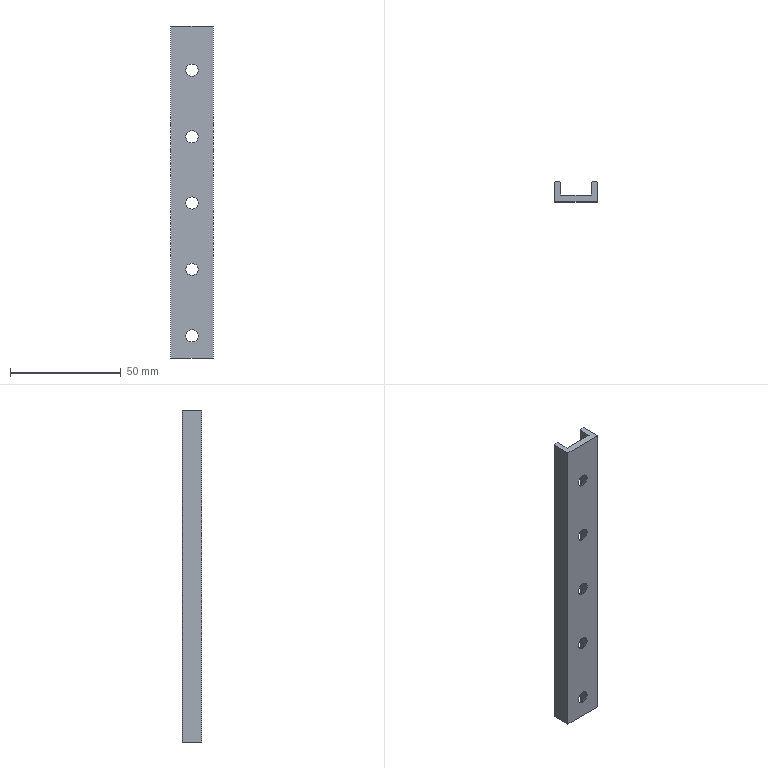Part | SolidWorks | features Chamfer 1, Extrusion 1, HoleWzd 1, LPattern 1 | 1 solid | 34 faces | box 19 x 9 x 150 mm | volume 12195 mm3 | plane 14 | cone 10 | cylinder 10 | commonest cylinder face diameters 5.5 x10
STEP:
#1=CARTESIAN_POINT('',(0.,-4.35,127.25));
#2=VERTEX_POINT('',#1);
#3=CARTESIAN_POINT('',(0.,-4.35,132.75));
#4=VERTEX_POINT('',#3);
#5=CARTESIAN_POINT('',(0.,-4.35,130.));
#6=DIRECTION('',(0.,1.,0.));
#7=DIRECTION('',(0.,0.,1.));
#8=AXIS2_PLACEMENT_3D('',#5,#6,#7);
#9=CIRCLE('',#8,2.75);
#10=EDGE_CURVE('',#2,#4,#9,.T.);
#11=ORIENTED_EDGE('',*,*,#10,.F.);
#12=CARTESIAN_POINT('',(0.,-1.5,124.4));
#13=VERTEX_POINT('',#12);
#14=CARTESIAN_POINT('',(0.,-1.5,124.4));
#15=DIRECTION('',(0.,0.7071,-0.7071));
#16=VECTOR('',#15,1000.);
#17=LINE('',#14,#16);
#18=EDGE_CURVE('',#2,#13,#17,.T.);
#19=ORIENTED_EDGE('',*,*,#18,.T.);
#20=CARTESIAN_POINT('',(0.,-1.5,135.6));
#21=VERTEX_POINT('',#20);
#22=CARTESIAN_POINT('',(0.,-1.5,130.));
#23=DIRECTION('',(0.,1.,0.));
#24=DIRECTION('',(0.,0.,1.));
#25=AXIS2_PLACEMENT_3D('',#22,#23,#24);
#26=CIRCLE('',#25,5.6);
#27=EDGE_CURVE('',#13,#21,#26,.T.);
#28=ORIENTED_EDGE('',*,*,#27,.T.);
#29=CARTESIAN_POINT('',(0.,-1.5,135.6));
#30=DIRECTION('',(0.,0.7071,0.7071));
#31=VECTOR('',#30,1000.);
#32=LINE('',#29,#31);
#33=EDGE_CURVE('',#4,#21,#32,.T.);
#34=ORIENTED_EDGE('',*,*,#33,.F.);
#35=EDGE_LOOP('',(#11,#19,#28,#34));
#36=FACE_OUTER_BOUND('',#35,.T.);
#37=CARTESIAN_POINT('',(0.,-1.5,130.));
#38=DIRECTION('',(0.,1.,0.));
#39=DIRECTION('',(0.,0.,1.));
#40=AXIS2_PLACEMENT_3D('',#37,#38,#39);
#41=CONICAL_SURFACE('',#40,5.6,0.7854);
#42=ADVANCED_FACE('',(#36),#41,.F.);
#43=CARTESIAN_POINT('',(0.,-4.5,127.25));
#44=VERTEX_POINT('',#43);
#45=CARTESIAN_POINT('',(0.,-4.5,132.75));
#46=VERTEX_POINT('',#45);
#47=CARTESIAN_POINT('',(0.,-4.5,130.));
#48=DIRECTION('',(0.,1.,0.));
#49=DIRECTION('',(0.,0.,1.));
#50=AXIS2_PLACEMENT_3D('',#47,#48,#49);
#51=CIRCLE('',#50,2.75);
#52=EDGE_CURVE('',#44,#46,#51,.T.);
#53=ORIENTED_EDGE('',*,*,#52,.F.);
#54=CARTESIAN_POINT('',(0.,-1.5,127.25));
#55=DIRECTION('',(0.,1.,0.));
#56=VECTOR('',#55,1000.);
#57=LINE('',#54,#56);
#58=EDGE_CURVE('',#44,#2,#57,.T.);
#59=ORIENTED_EDGE('',*,*,#58,.T.);
#60=ORIENTED_EDGE('',*,*,#10,.T.);
#61=CARTESIAN_POINT('',(0.,-1.5,132.75));
#62=DIRECTION('',(0.,1.,0.));
#63=VECTOR('',#62,1000.);
#64=LINE('',#61,#63);
#65=EDGE_CURVE('',#46,#4,#64,.T.);
#66=ORIENTED_EDGE('',*,*,#65,.F.);
#67=EDGE_LOOP('',(#53,#59,#60,#66));
#68=FACE_OUTER_BOUND('',#67,.T.);
#69=CARTESIAN_POINT('',(0.,-1.5,130.));
#70=DIRECTION('',(0.,1.,0.));
#71=DIRECTION('',(0.,0.,1.));
#72=AXIS2_PLACEMENT_3D('',#69,#70,#71);
#73=CYLINDRICAL_SURFACE('',#72,2.75);
#74=ADVANCED_FACE('',(#68),#73,.F.);
#75=CARTESIAN_POINT('',(0.,-4.35,97.25));
#76=VERTEX_POINT('',#75);
#77=CARTESIAN_POINT('',(0.,-4.35,102.75));
#78=VERTEX_POINT('',#77);
#79=CARTESIAN_POINT('',(0.,-4.35,100.));
#80=DIRECTION('',(0.,1.,0.));
#81=DIRECTION('',(0.,0.,1.));
#82=AXIS2_PLACEMENT_3D('',#79,#80,#81);
#83=CIRCLE('',#82,2.75);
#84=EDGE_CURVE('',#76,#78,#83,.T.);
#85=ORIENTED_EDGE('',*,*,#84,.F.);
#86=CARTESIAN_POINT('',(0.,-1.5,94.4));
#87=VERTEX_POINT('',#86);
#88=CARTESIAN_POINT('',(0.,-1.5,94.4));
#89=DIRECTION('',(0.,0.7071,-0.7071));
#90=VECTOR('',#89,1000.);
#91=LINE('',#88,#90);
#92=EDGE_CURVE('',#76,#87,#91,.T.);
#93=ORIENTED_EDGE('',*,*,#92,.T.);
#94=CARTESIAN_POINT('',(0.,-1.5,105.6));
#95=VERTEX_POINT('',#94);
#96=CARTESIAN_POINT('',(0.,-1.5,100.));
#97=DIRECTION('',(0.,1.,0.));
#98=DIRECTION('',(0.,0.,1.));
#99=AXIS2_PLACEMENT_3D('',#96,#97,#98);
#100=CIRCLE('',#99,5.6);
#101=EDGE_CURVE('',#87,#95,#100,.T.);
#102=ORIENTED_EDGE('',*,*,#101,.T.);
#103=CARTESIAN_POINT('',(0.,-1.5,105.6));
#104=DIRECTION('',(0.,0.7071,0.7071));
#105=VECTOR('',#104,1000.);
#106=LINE('',#103,#105);
#107=EDGE_CURVE('',#78,#95,#106,.T.);
#108=ORIENTED_EDGE('',*,*,#107,.F.);
#109=EDGE_LOOP('',(#85,#93,#102,#108));
#110=FACE_OUTER_BOUND('',#109,.T.);
#111=CARTESIAN_POINT('',(0.,-1.5,100.));
#112=DIRECTION('',(0.,1.,0.));
#113=DIRECTION('',(0.,0.,1.));
#114=AXIS2_PLACEMENT_3D('',#111,#112,#113);
#115=CONICAL_SURFACE('',#114,5.6,0.7854);
#116=ADVANCED_FACE('',(#110),#115,.F.);
#117=CARTESIAN_POINT('',(0.,-4.5,97.25));
#118=VERTEX_POINT('',#117);
#119=CARTESIAN_POINT('',(0.,-4.5,102.75));
#120=VERTEX_POINT('',#119);
#121=CARTESIAN_POINT('',(0.,-4.5,100.));
#122=DIRECTION('',(0.,1.,0.));
#123=DIRECTION('',(0.,0.,1.));
#124=AXIS2_PLACEMENT_3D('',#121,#122,#123);
#125=CIRCLE('',#124,2.75);
#126=EDGE_CURVE('',#118,#120,#125,.T.);
#127=ORIENTED_EDGE('',*,*,#126,.F.);
#128=CARTESIAN_POINT('',(0.,-1.5,97.25));
#129=DIRECTION('',(0.,1.,0.));
#130=VECTOR('',#129,1000.);
#131=LINE('',#128,#130);
#132=EDGE_CURVE('',#118,#76,#131,.T.);
#133=ORIENTED_EDGE('',*,*,#132,.T.);
#134=ORIENTED_EDGE('',*,*,#84,.T.);
#135=CARTESIAN_POINT('',(0.,-1.5,102.75));
#136=DIRECTION('',(0.,1.,0.));
#137=VECTOR('',#136,1000.);
#138=LINE('',#135,#137);
#139=EDGE_CURVE('',#120,#78,#138,.T.);
#140=ORIENTED_EDGE('',*,*,#139,.F.);
#141=EDGE_LOOP('',(#127,#133,#134,#140));
#142=FACE_OUTER_BOUND('',#141,.T.);
#143=CARTESIAN_POINT('',(0.,-1.5,100.));
#144=DIRECTION('',(0.,1.,0.));
#145=DIRECTION('',(0.,0.,1.));
#146=AXIS2_PLACEMENT_3D('',#143,#144,#145);
#147=CYLINDRICAL_SURFACE('',#146,2.75);
#148=ADVANCED_FACE('',(#142),#147,.F.);
#149=CARTESIAN_POINT('',(0.,-4.35,67.25));
#150=VERTEX_POINT('',#149);
#151=CARTESIAN_POINT('',(0.,-4.35,72.75));
#152=VERTEX_POINT('',#151);
#153=CARTESIAN_POINT('',(0.,-4.35,70.));
#154=DIRECTION('',(0.,1.,0.));
#155=DIRECTION('',(0.,0.,1.));
#156=AXIS2_PLACEMENT_3D('',#153,#154,#155);
#157=CIRCLE('',#156,2.75);
#158=EDGE_CURVE('',#150,#152,#157,.T.);
#159=ORIENTED_EDGE('',*,*,#158,.F.);
#160=CARTESIAN_POINT('',(0.,-1.5,64.4));
#161=VERTEX_POINT('',#160);
#162=CARTESIAN_POINT('',(0.,-1.5,64.4));
#163=DIRECTION('',(0.,0.7071,-0.7071));
#164=VECTOR('',#163,1000.);
#165=LINE('',#162,#164);
#166=EDGE_CURVE('',#150,#161,#165,.T.);
#167=ORIENTED_EDGE('',*,*,#166,.T.);
#168=CARTESIAN_POINT('',(0.,-1.5,75.6));
#169=VERTEX_POINT('',#168);
#170=CARTESIAN_POINT('',(0.,-1.5,70.));
#171=DIRECTION('',(0.,1.,0.));
#172=DIRECTION('',(0.,0.,1.));
#173=AXIS2_PLACEMENT_3D('',#170,#171,#172);
#174=CIRCLE('',#173,5.6);
#175=EDGE_CURVE('',#161,#169,#174,.T.);
#176=ORIENTED_EDGE('',*,*,#175,.T.);
#177=CARTESIAN_POINT('',(0.,-1.5,75.6));
#178=DIRECTION('',(0.,0.7071,0.7071));
#179=VECTOR('',#178,1000.);
#180=LINE('',#177,#179);
#181=EDGE_CURVE('',#152,#169,#180,.T.);
#182=ORIENTED_EDGE('',*,*,#181,.F.);
#183=EDGE_LOOP('',(#159,#167,#176,#182));
#184=FACE_OUTER_BOUND('',#183,.T.);
#185=CARTESIAN_POINT('',(0.,-1.5,70.));
#186=DIRECTION('',(0.,1.,0.));
#187=DIRECTION('',(0.,0.,1.));
#188=AXIS2_PLACEMENT_3D('',#185,#186,#187);
#189=CONICAL_SURFACE('',#188,5.6,0.7854);
#190=ADVANCED_FACE('',(#184),#189,.F.);
#191=CARTESIAN_POINT('',(0.,-4.5,67.25));
#192=VERTEX_POINT('',#191);
#193=CARTESIAN_POINT('',(0.,-4.5,72.75));
#194=VERTEX_POINT('',#193);
#195=CARTESIAN_POINT('',(0.,-4.5,70.));
#196=DIRECTION('',(0.,1.,0.));
#197=DIRECTION('',(0.,0.,1.));
#198=AXIS2_PLACEMENT_3D('',#195,#196,#197);
#199=CIRCLE('',#198,2.75);
#200=EDGE_CURVE('',#192,#194,#199,.T.);
#201=ORIENTED_EDGE('',*,*,#200,.F.);
#202=CARTESIAN_POINT('',(0.,-1.5,67.25));
#203=DIRECTION('',(0.,1.,0.));
#204=VECTOR('',#203,1000.);
#205=LINE('',#202,#204);
#206=EDGE_CURVE('',#192,#150,#205,.T.);
#207=ORIENTED_EDGE('',*,*,#206,.T.);
#208=ORIENTED_EDGE('',*,*,#158,.T.);
#209=CARTESIAN_POINT('',(0.,-1.5,72.75));
#210=DIRECTION('',(0.,1.,0.));
#211=VECTOR('',#210,1000.);
#212=LINE('',#209,#211);
#213=EDGE_CURVE('',#194,#152,#212,.T.);
#214=ORIENTED_EDGE('',*,*,#213,.F.);
#215=EDGE_LOOP('',(#201,#207,#208,#214));
#216=FACE_OUTER_BOUND('',#215,.T.);
#217=CARTESIAN_POINT('',(0.,-1.5,70.));
#218=DIRECTION('',(0.,1.,0.));
#219=DIRECTION('',(0.,0.,1.));
#220=AXIS2_PLACEMENT_3D('',#217,#218,#219);
#221=CYLINDRICAL_SURFACE('',#220,2.75);
#222=ADVANCED_FACE('',(#216),#221,.F.);
#223=CARTESIAN_POINT('',(0.,-4.35,7.25));
#224=VERTEX_POINT('',#223);
#225=CARTESIAN_POINT('',(0.,-4.35,12.75));
#226=VERTEX_POINT('',#225);
#227=CARTESIAN_POINT('',(0.,-4.35,10.));
#228=DIRECTION('',(0.,1.,0.));
#229=DIRECTION('',(0.,0.,1.));
#230=AXIS2_PLACEMENT_3D('',#227,#228,#229);
#231=CIRCLE('',#230,2.75);
#232=EDGE_CURVE('',#224,#226,#231,.T.);
#233=ORIENTED_EDGE('',*,*,#232,.F.);
#234=CARTESIAN_POINT('',(0.,-1.5,4.4));
#235=VERTEX_POINT('',#234);
#236=CARTESIAN_POINT('',(0.,-1.5,4.4));
#237=DIRECTION('',(0.,0.7071,-0.7071));
#238=VECTOR('',#237,1000.);
#239=LINE('',#236,#238);
#240=EDGE_CURVE('',#224,#235,#239,.T.);
#241=ORIENTED_EDGE('',*,*,#240,.T.);
#242=CARTESIAN_POINT('',(0.,-1.5,15.6));
#243=VERTEX_POINT('',#242);
#244=CARTESIAN_POINT('',(0.,-1.5,10.));
#245=DIRECTION('',(0.,1.,0.));
#246=DIRECTION('',(0.,0.,1.));
#247=AXIS2_PLACEMENT_3D('',#244,#245,#246);
#248=CIRCLE('',#247,5.6);
#249=EDGE_CURVE('',#235,#243,#248,.T.);
#250=ORIENTED_EDGE('',*,*,#249,.T.);
#251=CARTESIAN_POINT('',(0.,-1.5,15.6));
#252=DIRECTION('',(0.,0.7071,0.7071));
#253=VECTOR('',#252,1000.);
#254=LINE('',#251,#253);
#255=EDGE_CURVE('',#226,#243,#254,.T.);
#256=ORIENTED_EDGE('',*,*,#255,.F.);
#257=EDGE_LOOP('',(#233,#241,#250,#256));
#258=FACE_OUTER_BOUND('',#257,.T.);
#259=CARTESIAN_POINT('',(0.,-1.5,10.));
#260=DIRECTION('',(0.,1.,0.));
#261=DIRECTION('',(0.,0.,1.));
#262=AXIS2_PLACEMENT_3D('',#259,#260,#261);
#263=CONICAL_SURFACE('',#262,5.6,0.7854);
#264=ADVANCED_FACE('',(#258),#263,.F.);
#265=CARTESIAN_POINT('',(0.,-4.5,7.25));
#266=VERTEX_POINT('',#265);
#267=CARTESIAN_POINT('',(0.,-4.5,12.75));
#268=VERTEX_POINT('',#267);
#269=CARTESIAN_POINT('',(0.,-4.5,10.));
#270=DIRECTION('',(0.,1.,0.));
#271=DIRECTION('',(0.,0.,1.));
#272=AXIS2_PLACEMENT_3D('',#269,#270,#271);
#273=CIRCLE('',#272,2.75);
#274=EDGE_CURVE('',#266,#268,#273,.T.);
#275=ORIENTED_EDGE('',*,*,#274,.F.);
#276=CARTESIAN_POINT('',(0.,-1.5,7.25));
#277=DIRECTION('',(0.,1.,0.));
#278=VECTOR('',#277,1000.);
#279=LINE('',#276,#278);
#280=EDGE_CURVE('',#266,#224,#279,.T.);
#281=ORIENTED_EDGE('',*,*,#280,.T.);
#282=ORIENTED_EDGE('',*,*,#232,.T.);
#283=CARTESIAN_POINT('',(0.,-1.5,12.75));
#284=DIRECTION('',(0.,1.,0.));
#285=VECTOR('',#284,1000.);
#286=LINE('',#283,#285);
#287=EDGE_CURVE('',#268,#226,#286,.T.);
#288=ORIENTED_EDGE('',*,*,#287,.F.);
#289=EDGE_LOOP('',(#275,#281,#282,#288));
#290=FACE_OUTER_BOUND('',#289,.T.);
#291=CARTESIAN_POINT('',(0.,-1.5,10.));
#292=DIRECTION('',(0.,1.,0.));
#293=DIRECTION('',(0.,0.,1.));
#294=AXIS2_PLACEMENT_3D('',#291,#292,#293);
#295=CYLINDRICAL_SURFACE('',#294,2.75);
#296=ADVANCED_FACE('',(#290),#295,.F.);
#297=CARTESIAN_POINT('',(0.,-4.35,37.25));
#298=VERTEX_POINT('',#297);
#299=CARTESIAN_POINT('',(0.,-4.35,42.75));
#300=VERTEX_POINT('',#299);
#301=CARTESIAN_POINT('',(0.,-4.35,40.));
#302=DIRECTION('',(0.,1.,0.));
#303=DIRECTION('',(0.,0.,1.));
#304=AXIS2_PLACEMENT_3D('',#301,#302,#303);
#305=CIRCLE('',#304,2.75);
#306=EDGE_CURVE('',#298,#300,#305,.T.);
#307=ORIENTED_EDGE('',*,*,#306,.F.);
#308=CARTESIAN_POINT('',(0.,-1.5,34.4));
#309=VERTEX_POINT('',#308);
#310=CARTESIAN_POINT('',(0.,-1.5,34.4));
#311=DIRECTION('',(0.,0.7071,-0.7071));
#312=VECTOR('',#311,1000.);
#313=LINE('',#310,#312);
#314=EDGE_CURVE('',#298,#309,#313,.T.);
#315=ORIENTED_EDGE('',*,*,#314,.T.);
#316=CARTESIAN_POINT('',(0.,-1.5,45.6));
#317=VERTEX_POINT('',#316);
#318=CARTESIAN_POINT('',(0.,-1.5,40.));
#319=DIRECTION('',(0.,1.,0.));
#320=DIRECTION('',(0.,0.,1.));
#321=AXIS2_PLACEMENT_3D('',#318,#319,#320);
#322=CIRCLE('',#321,5.6);
#323=EDGE_CURVE('',#309,#317,#322,.T.);
#324=ORIENTED_EDGE('',*,*,#323,.T.);
#325=CARTESIAN_POINT('',(0.,-1.5,45.6));
#326=DIRECTION('',(0.,0.7071,0.7071));
#327=VECTOR('',#326,1000.);
#328=LINE('',#325,#327);
#329=EDGE_CURVE('',#300,#317,#328,.T.);
#330=ORIENTED_EDGE('',*,*,#329,.F.);
#331=EDGE_LOOP('',(#307,#315,#324,#330));
#332=FACE_OUTER_BOUND('',#331,.T.);
#333=CARTESIAN_POINT('',(0.,-1.5,40.));
#334=DIRECTION('',(0.,1.,0.));
#335=DIRECTION('',(0.,0.,1.));
#336=AXIS2_PLACEMENT_3D('',#333,#334,#335);
#337=CONICAL_SURFACE('',#336,5.6,0.7854);
#338=ADVANCED_FACE('',(#332),#337,.F.);
#339=CARTESIAN_POINT('',(0.,-4.5,37.25));
#340=VERTEX_POINT('',#339);
#341=CARTESIAN_POINT('',(0.,-4.5,42.75));
#342=VERTEX_POINT('',#341);
#343=CARTESIAN_POINT('',(0.,-4.5,40.));
#344=DIRECTION('',(0.,1.,0.));
#345=DIRECTION('',(0.,0.,1.));
#346=AXIS2_PLACEMENT_3D('',#343,#344,#345);
#347=CIRCLE('',#346,2.75);
#348=EDGE_CURVE('',#340,#342,#347,.T.);
#349=ORIENTED_EDGE('',*,*,#348,.F.);
#350=CARTESIAN_POINT('',(0.,-1.5,37.25));
#351=DIRECTION('',(0.,1.,0.));
#352=VECTOR('',#351,1000.);
#353=LINE('',#350,#352);
#354=EDGE_CURVE('',#340,#298,#353,.T.);
#355=ORIENTED_EDGE('',*,*,#354,.T.);
#356=ORIENTED_EDGE('',*,*,#306,.T.);
#357=CARTESIAN_POINT('',(0.,-1.5,42.75));
#358=DIRECTION('',(0.,1.,0.));
#359=VECTOR('',#358,1000.);
#360=LINE('',#357,#359);
#361=EDGE_CURVE('',#342,#300,#360,.T.);
#362=ORIENTED_EDGE('',*,*,#361,.F.);
#363=EDGE_LOOP('',(#349,#355,#356,#362));
#364=FACE_OUTER_BOUND('',#363,.T.);
#365=CARTESIAN_POINT('',(0.,-1.5,40.));
#366=DIRECTION('',(0.,1.,0.));
#367=DIRECTION('',(0.,0.,1.));
#368=AXIS2_PLACEMENT_3D('',#365,#366,#367);
#369=CYLINDRICAL_SURFACE('',#368,2.75);
#370=ADVANCED_FACE('',(#364),#369,.F.);
#371=CARTESIAN_POINT('',(9.2,4.5,150.));
#372=VERTEX_POINT('',#371);
#373=CARTESIAN_POINT('',(7.3,4.5,150.));
#374=VERTEX_POINT('',#373);
#375=CARTESIAN_POINT('',(7.,4.5,150.));
#376=DIRECTION('',(-1.,0.,0.));
#377=VECTOR('',#376,1000.);
#378=LINE('',#375,#377);
#379=EDGE_CURVE('',#372,#374,#378,.T.);
#380=ORIENTED_EDGE('',*,*,#379,.F.);
#381=CARTESIAN_POINT('',(9.2,4.5,0.));
#382=VERTEX_POINT('',#381);
#383=CARTESIAN_POINT('',(9.2,4.5,150.));
#384=DIRECTION('',(0.,0.,-1.));
#385=VECTOR('',#384,1000.);
#386=LINE('',#383,#385);
#387=EDGE_CURVE('',#372,#382,#386,.T.);
#388=ORIENTED_EDGE('',*,*,#387,.T.);
#389=CARTESIAN_POINT('',(7.3,4.5,0.));
#390=VERTEX_POINT('',#389);
#391=CARTESIAN_POINT('',(7.,4.5,0.));
#392=DIRECTION('',(-1.,0.,0.));
#393=VECTOR('',#392,1000.);
#394=LINE('',#391,#393);
#395=EDGE_CURVE('',#382,#390,#394,.T.);
#396=ORIENTED_EDGE('',*,*,#395,.T.);
#397=CARTESIAN_POINT('',(7.3,4.5,150.));
#398=DIRECTION('',(0.,0.,1.));
#399=VECTOR('',#398,1000.);
#400=LINE('',#397,#399);
#401=EDGE_CURVE('',#390,#374,#400,.T.);
#402=ORIENTED_EDGE('',*,*,#401,.T.);
#403=EDGE_LOOP('',(#380,#388,#396,#402));
#404=FACE_OUTER_BOUND('',#403,.T.);
#405=CARTESIAN_POINT('',(7.,4.5,150.));
#406=DIRECTION('',(0.,-1.,0.));
#407=DIRECTION('',(1.,0.,0.));
#408=AXIS2_PLACEMENT_3D('',#405,#406,#407);
#409=PLANE('',#408);
#410=ADVANCED_FACE('',(#404),#409,.F.);
#411=CARTESIAN_POINT('',(7.,4.2,150.));
#412=VERTEX_POINT('',#411);
#413=CARTESIAN_POINT('',(7.,-1.5,150.));
#414=VERTEX_POINT('',#413);
#415=CARTESIAN_POINT('',(7.,-1.5,150.));
#416=DIRECTION('',(0.,-1.,0.));
#417=VECTOR('',#416,1000.);
#418=LINE('',#415,#417);
#419=EDGE_CURVE('',#412,#414,#418,.T.);
#420=ORIENTED_EDGE('',*,*,#419,.F.);
#421=CARTESIAN_POINT('',(7.,4.2,0.));
#422=VERTEX_POINT('',#421);
#423=CARTESIAN_POINT('',(7.,4.2,150.));
#424=DIRECTION('',(0.,0.,-1.));
#425=VECTOR('',#424,1000.);
#426=LINE('',#423,#425);
#427=EDGE_CURVE('',#412,#422,#426,.T.);
#428=ORIENTED_EDGE('',*,*,#427,.T.);
#429=CARTESIAN_POINT('',(7.,-1.5,0.));
#430=VERTEX_POINT('',#429);
#431=CARTESIAN_POINT('',(7.,-1.5,0.));
#432=DIRECTION('',(0.,-1.,0.));
#433=VECTOR('',#432,1000.);
#434=LINE('',#431,#433);
#435=EDGE_CURVE('',#422,#430,#434,.T.);
#436=ORIENTED_EDGE('',*,*,#435,.T.);
#437=CARTESIAN_POINT('',(7.,-1.5,150.));
#438=DIRECTION('',(0.,0.,-1.));
#439=VECTOR('',#438,1000.);
#440=LINE('',#437,#439);
#441=EDGE_CURVE('',#414,#430,#440,.T.);
#442=ORIENTED_EDGE('',*,*,#441,.F.);
#443=EDGE_LOOP('',(#420,#428,#436,#442));
#444=FACE_OUTER_BOUND('',#443,.T.);
#445=CARTESIAN_POINT('',(7.,-1.5,150.));
#446=DIRECTION('',(1.,0.,0.));
#447=DIRECTION('',(0.,1.,0.));
#448=AXIS2_PLACEMENT_3D('',#445,#446,#447);
#449=PLANE('',#448);
#450=ADVANCED_FACE('',(#444),#449,.F.);
#451=CARTESIAN_POINT('',(0.,-1.5,130.));
#452=DIRECTION('',(0.,1.,0.));
#453=DIRECTION('',(0.,0.,1.));
#454=AXIS2_PLACEMENT_3D('',#451,#452,#453);
#455=CIRCLE('',#454,5.6);
#456=EDGE_CURVE('',#21,#13,#455,.T.);
#457=ORIENTED_EDGE('',*,*,#456,.F.);
#458=ORIENTED_EDGE('',*,*,#27,.F.);
#459=EDGE_LOOP('',(#457,#458));
#460=FACE_BOUND('',#459,.T.);
#461=CARTESIAN_POINT('',(0.,-1.5,100.));
#462=DIRECTION('',(0.,1.,0.));
#463=DIRECTION('',(0.,0.,1.));
#464=AXIS2_PLACEMENT_3D('',#461,#462,#463);
#465=CIRCLE('',#464,5.6);
#466=EDGE_CURVE('',#95,#87,#465,.T.);
#467=ORIENTED_EDGE('',*,*,#466,.F.);
#468=ORIENTED_EDGE('',*,*,#101,.F.);
#469=EDGE_LOOP('',(#467,#468));
#470=FACE_BOUND('',#469,.T.);
#471=CARTESIAN_POINT('',(0.,-1.5,70.));
#472=DIRECTION('',(0.,1.,0.));
#473=DIRECTION('',(0.,0.,1.));
#474=AXIS2_PLACEMENT_3D('',#471,#472,#473);
#475=CIRCLE('',#474,5.6);
#476=EDGE_CURVE('',#169,#161,#475,.T.);
#477=ORIENTED_EDGE('',*,*,#476,.F.);
#478=ORIENTED_EDGE('',*,*,#175,.F.);
#479=EDGE_LOOP('',(#477,#478));
#480=FACE_BOUND('',#479,.T.);
#481=CARTESIAN_POINT('',(0.,-1.5,10.));
#482=DIRECTION('',(0.,1.,0.));
#483=DIRECTION('',(0.,0.,1.));
#484=AXIS2_PLACEMENT_3D('',#481,#482,#483);
#485=CIRCLE('',#484,5.6);
#486=EDGE_CURVE('',#243,#235,#485,.T.);
#487=ORIENTED_EDGE('',*,*,#486,.F.);
#488=ORIENTED_EDGE('',*,*,#249,.F.);
#489=EDGE_LOOP('',(#487,#488));
#490=FACE_BOUND('',#489,.T.);
#491=CARTESIAN_POINT('',(0.,-1.5,40.));
#492=DIRECTION('',(0.,1.,0.));
#493=DIRECTION('',(0.,0.,1.));
#494=AXIS2_PLACEMENT_3D('',#491,#492,#493);
#495=CIRCLE('',#494,5.6);
#496=EDGE_CURVE('',#317,#309,#495,.T.);
#497=ORIENTED_EDGE('',*,*,#496,.F.);
#498=ORIENTED_EDGE('',*,*,#323,.F.);
#499=EDGE_LOOP('',(#497,#498));
#500=FACE_BOUND('',#499,.T.);
#501=CARTESIAN_POINT('',(-7.,-1.5,0.));
#502=VERTEX_POINT('',#501);
#503=CARTESIAN_POINT('',(-7.,-1.5,0.));
#504=DIRECTION('',(-1.,0.,0.));
#505=VECTOR('',#504,1000.);
#506=LINE('',#503,#505);
#507=EDGE_CURVE('',#430,#502,#506,.T.);
#508=ORIENTED_EDGE('',*,*,#507,.T.);
#509=CARTESIAN_POINT('',(-7.,-1.5,150.));
#510=VERTEX_POINT('',#509);
#511=CARTESIAN_POINT('',(-7.,-1.5,150.));
#512=DIRECTION('',(0.,0.,-1.));
#513=VECTOR('',#512,1000.);
#514=LINE('',#511,#513);
#515=EDGE_CURVE('',#510,#502,#514,.T.);
#516=ORIENTED_EDGE('',*,*,#515,.F.);
#517=CARTESIAN_POINT('',(-7.,-1.5,150.));
#518=DIRECTION('',(-1.,0.,0.));
#519=VECTOR('',#518,1000.);
#520=LINE('',#517,#519);
#521=EDGE_CURVE('',#414,#510,#520,.T.);
#522=ORIENTED_EDGE('',*,*,#521,.F.);
#523=ORIENTED_EDGE('',*,*,#441,.T.);
#524=EDGE_LOOP('',(#508,#516,#522,#523));
#525=FACE_OUTER_BOUND('',#524,.T.);
#526=CARTESIAN_POINT('',(-7.,-1.5,150.));
#527=DIRECTION('',(0.,-1.,0.));
#528=DIRECTION('',(1.,0.,0.));
#529=AXIS2_PLACEMENT_3D('',#526,#527,#528);
#530=PLANE('',#529);
#531=ADVANCED_FACE('',(#460,#470,#480,#490,#500,#525),#530,.F.);
#532=CARTESIAN_POINT('',(-7.,4.2,0.));
#533=VERTEX_POINT('',#532);
#534=CARTESIAN_POINT('',(-7.,4.5,0.));
#535=DIRECTION('',(0.,1.,0.));
#536=VECTOR('',#535,1000.);
#537=LINE('',#534,#536);
#538=EDGE_CURVE('',#502,#533,#537,.T.);
#539=ORIENTED_EDGE('',*,*,#538,.T.);
#540=CARTESIAN_POINT('',(-7.,4.2,150.));
#541=VERTEX_POINT('',#540);
#542=CARTESIAN_POINT('',(-7.,4.2,150.));
#543=DIRECTION('',(0.,0.,1.));
#544=VECTOR('',#543,1000.);
#545=LINE('',#542,#544);
#546=EDGE_CURVE('',#533,#541,#545,.T.);
#547=ORIENTED_EDGE('',*,*,#546,.T.);
#548=CARTESIAN_POINT('',(-7.,4.5,150.));
#549=DIRECTION('',(0.,1.,0.));
#550=VECTOR('',#549,1000.);
#551=LINE('',#548,#550);
#552=EDGE_CURVE('',#510,#541,#551,.T.);
#553=ORIENTED_EDGE('',*,*,#552,.F.);
#554=ORIENTED_EDGE('',*,*,#515,.T.);
#555=EDGE_LOOP('',(#539,#547,#553,#554));
#556=FACE_OUTER_BOUND('',#555,.T.);
#557=CARTESIAN_POINT('',(-7.,4.5,150.));
#558=DIRECTION('',(-1.,0.,0.));
#559=DIRECTION('',(0.,-1.,0.));
#560=AXIS2_PLACEMENT_3D('',#557,#558,#559);
#561=PLANE('',#560);
#562=ADVANCED_FACE('',(#556),#561,.F.);
#563=CARTESIAN_POINT('',(-7.3,4.5,0.));
#564=VERTEX_POINT('',#563);
#565=CARTESIAN_POINT('',(-9.2,4.5,0.));
#566=VERTEX_POINT('',#565);
#567=CARTESIAN_POINT('',(-9.5,4.5,0.));
#568=DIRECTION('',(-1.,0.,0.));
#569=VECTOR('',#568,1000.);
#570=LINE('',#567,#569);
#571=EDGE_CURVE('',#564,#566,#570,.T.);
#572=ORIENTED_EDGE('',*,*,#571,.T.);
#573=CARTESIAN_POINT('',(-9.2,4.5,150.));
#574=VERTEX_POINT('',#573);
#575=CARTESIAN_POINT('',(-9.2,4.5,150.));
#576=DIRECTION('',(0.,0.,1.));
#577=VECTOR('',#576,1000.);
#578=LINE('',#575,#577);
#579=EDGE_CURVE('',#566,#574,#578,.T.);
#580=ORIENTED_EDGE('',*,*,#579,.T.);
#581=CARTESIAN_POINT('',(-7.3,4.5,150.));
#582=VERTEX_POINT('',#581);
#583=CARTESIAN_POINT('',(-9.5,4.5,150.));
#584=DIRECTION('',(-1.,0.,0.));
#585=VECTOR('',#584,1000.);
#586=LINE('',#583,#585);
#587=EDGE_CURVE('',#582,#574,#586,.T.);
#588=ORIENTED_EDGE('',*,*,#587,.F.);
#589=CARTESIAN_POINT('',(-7.3,4.5,150.));
#590=DIRECTION('',(0.,0.,-1.));
#591=VECTOR('',#590,1000.);
#592=LINE('',#589,#591);
#593=EDGE_CURVE('',#582,#564,#592,.T.);
#594=ORIENTED_EDGE('',*,*,#593,.T.);
#595=EDGE_LOOP('',(#572,#580,#588,#594));
#596=FACE_OUTER_BOUND('',#595,.T.);
#597=CARTESIAN_POINT('',(-9.5,4.5,150.));
#598=DIRECTION('',(0.,-1.,0.));
#599=DIRECTION('',(1.,0.,0.));
#600=AXIS2_PLACEMENT_3D('',#597,#598,#599);
#601=PLANE('',#600);
#602=ADVANCED_FACE('',(#596),#601,.F.);
#603=CARTESIAN_POINT('',(-9.5,4.2,150.));
#604=VERTEX_POINT('',#603);
#605=CARTESIAN_POINT('',(-9.5,-4.5,150.));
#606=VERTEX_POINT('',#605);
#607=CARTESIAN_POINT('',(-9.5,-4.5,150.));
#608=DIRECTION('',(0.,-1.,0.));
#609=VECTOR('',#608,1000.);
#610=LINE('',#607,#609);
#611=EDGE_CURVE('',#604,#606,#610,.T.);
#612=ORIENTED_EDGE('',*,*,#611,.F.);
#613=CARTESIAN_POINT('',(-9.5,4.2,0.));
#614=VERTEX_POINT('',#613);
#615=CARTESIAN_POINT('',(-9.5,4.2,150.));
#616=DIRECTION('',(0.,0.,-1.));
#617=VECTOR('',#616,1000.);
#618=LINE('',#615,#617);
#619=EDGE_CURVE('',#604,#614,#618,.T.);
#620=ORIENTED_EDGE('',*,*,#619,.T.);
#621=CARTESIAN_POINT('',(-9.5,-4.5,0.));
#622=VERTEX_POINT('',#621);
#623=CARTESIAN_POINT('',(-9.5,-4.5,0.));
#624=DIRECTION('',(0.,-1.,0.));
#625=VECTOR('',#624,1000.);
#626=LINE('',#623,#625);
#627=EDGE_CURVE('',#614,#622,#626,.T.);
#628=ORIENTED_EDGE('',*,*,#627,.T.);
#629=CARTESIAN_POINT('',(-9.5,-4.5,150.));
#630=DIRECTION('',(0.,0.,-1.));
#631=VECTOR('',#630,1000.);
#632=LINE('',#629,#631);
#633=EDGE_CURVE('',#606,#622,#632,.T.);
#634=ORIENTED_EDGE('',*,*,#633,.F.);
#635=EDGE_LOOP('',(#612,#620,#628,#634));
#636=FACE_OUTER_BOUND('',#635,.T.);
#637=CARTESIAN_POINT('',(-9.5,-4.5,150.));
#638=DIRECTION('',(1.,0.,0.));
#639=DIRECTION('',(0.,0.,-1.));
#640=AXIS2_PLACEMENT_3D('',#637,#638,#639);
#641=PLANE('',#640);
#642=ADVANCED_FACE('',(#636),#641,.F.);
#643=CARTESIAN_POINT('',(0.,-4.5,130.));
#644=DIRECTION('',(0.,1.,0.));
#645=DIRECTION('',(0.,0.,1.));
#646=AXIS2_PLACEMENT_3D('',#643,#644,#645);
#647=CIRCLE('',#646,2.75);
#648=EDGE_CURVE('',#46,#44,#647,.T.);
#649=ORIENTED_EDGE('',*,*,#648,.T.);
#650=ORIENTED_EDGE('',*,*,#52,.T.);
#651=EDGE_LOOP('',(#649,#650));
#652=FACE_BOUND('',#651,.T.);
#653=CARTESIAN_POINT('',(0.,-4.5,100.));
#654=DIRECTION('',(0.,1.,0.));
#655=DIRECTION('',(0.,0.,1.));
#656=AXIS2_PLACEMENT_3D('',#653,#654,#655);
#657=CIRCLE('',#656,2.75);
#658=EDGE_CURVE('',#120,#118,#657,.T.);
#659=ORIENTED_EDGE('',*,*,#658,.T.);
#660=ORIENTED_EDGE('',*,*,#126,.T.);
#661=EDGE_LOOP('',(#659,#660));
#662=FACE_BOUND('',#661,.T.);
#663=CARTESIAN_POINT('',(0.,-4.5,70.));
#664=DIRECTION('',(0.,1.,0.));
#665=DIRECTION('',(0.,0.,1.));
#666=AXIS2_PLACEMENT_3D('',#663,#664,#665);
#667=CIRCLE('',#666,2.75);
#668=EDGE_CURVE('',#194,#192,#667,.T.);
#669=ORIENTED_EDGE('',*,*,#668,.T.);
#670=ORIENTED_EDGE('',*,*,#200,.T.);
#671=EDGE_LOOP('',(#669,#670));
#672=FACE_BOUND('',#671,.T.);
#673=CARTESIAN_POINT('',(0.,-4.5,10.));
#674=DIRECTION('',(0.,1.,0.));
#675=DIRECTION('',(0.,0.,1.));
#676=AXIS2_PLACEMENT_3D('',#673,#674,#675);
#677=CIRCLE('',#676,2.75);
#678=EDGE_CURVE('',#268,#266,#677,.T.);
#679=ORIENTED_EDGE('',*,*,#678,.T.);
#680=ORIENTED_EDGE('',*,*,#274,.T.);
#681=EDGE_LOOP('',(#679,#680));
#682=FACE_BOUND('',#681,.T.);
#683=CARTESIAN_POINT('',(0.,-4.5,40.));
#684=DIRECTION('',(0.,1.,0.));
#685=DIRECTION('',(0.,0.,1.));
#686=AXIS2_PLACEMENT_3D('',#683,#684,#685);
#687=CIRCLE('',#686,2.75);
#688=EDGE_CURVE('',#342,#340,#687,.T.);
#689=ORIENTED_EDGE('',*,*,#688,.T.);
#690=ORIENTED_EDGE('',*,*,#348,.T.);
#691=EDGE_LOOP('',(#689,#690));
#692=FACE_BOUND('',#691,.T.);
#693=CARTESIAN_POINT('',(9.5,-4.5,0.));
#694=VERTEX_POINT('',#693);
#695=CARTESIAN_POINT('',(-9.5,-4.5,0.));
#696=DIRECTION('',(1.,0.,0.));
#697=VECTOR('',#696,1000.);
#698=LINE('',#695,#697);
#699=EDGE_CURVE('',#622,#694,#698,.T.);
#700=ORIENTED_EDGE('',*,*,#699,.T.);
#701=CARTESIAN_POINT('',(9.5,-4.5,150.));
#702=VERTEX_POINT('',#701);
#703=CARTESIAN_POINT('',(9.5,-4.5,150.));
#704=DIRECTION('',(0.,0.,-1.));
#705=VECTOR('',#704,1000.);
#706=LINE('',#703,#705);
#707=EDGE_CURVE('',#702,#694,#706,.T.);
#708=ORIENTED_EDGE('',*,*,#707,.F.);
#709=CARTESIAN_POINT('',(-9.5,-4.5,150.));
#710=DIRECTION('',(1.,0.,0.));
#711=VECTOR('',#710,1000.);
#712=LINE('',#709,#711);
#713=EDGE_CURVE('',#606,#702,#712,.T.);
#714=ORIENTED_EDGE('',*,*,#713,.F.);
#715=ORIENTED_EDGE('',*,*,#633,.T.);
#716=EDGE_LOOP('',(#700,#708,#714,#715));
#717=FACE_OUTER_BOUND('',#716,.T.);
#718=CARTESIAN_POINT('',(-9.5,-4.5,150.));
#719=DIRECTION('',(0.,1.,0.));
#720=DIRECTION('',(0.,0.,1.));
#721=AXIS2_PLACEMENT_3D('',#718,#719,#720);
#722=PLANE('',#721);
#723=ADVANCED_FACE('',(#652,#662,#672,#682,#692,#717),#722,.F.);
#724=CARTESIAN_POINT('',(9.5,4.2,0.));
#725=VERTEX_POINT('',#724);
#726=CARTESIAN_POINT('',(9.5,-4.5,0.));
#727=DIRECTION('',(0.,1.,0.));
#728=VECTOR('',#727,1000.);
#729=LINE('',#726,#728);
#730=EDGE_CURVE('',#694,#725,#729,.T.);
#731=ORIENTED_EDGE('',*,*,#730,.T.);
#732=CARTESIAN_POINT('',(9.5,4.2,150.));
#733=VERTEX_POINT('',#732);
#734=CARTESIAN_POINT('',(9.5,4.2,150.));
#735=DIRECTION('',(0.,0.,1.));
#736=VECTOR('',#735,1000.);
#737=LINE('',#734,#736);
#738=EDGE_CURVE('',#725,#733,#737,.T.);
#739=ORIENTED_EDGE('',*,*,#738,.T.);
#740=CARTESIAN_POINT('',(9.5,-4.5,150.));
#741=DIRECTION('',(0.,1.,0.));
#742=VECTOR('',#741,1000.);
#743=LINE('',#740,#742);
#744=EDGE_CURVE('',#702,#733,#743,.T.);
#745=ORIENTED_EDGE('',*,*,#744,.F.);
#746=ORIENTED_EDGE('',*,*,#707,.T.);
#747=EDGE_LOOP('',(#731,#739,#745,#746));
#748=FACE_OUTER_BOUND('',#747,.T.);
#749=CARTESIAN_POINT('',(9.5,-4.5,150.));
#750=DIRECTION('',(-1.,0.,0.));
#751=DIRECTION('',(0.,0.,1.));
#752=AXIS2_PLACEMENT_3D('',#749,#750,#751);
#753=PLANE('',#752);
#754=ADVANCED_FACE('',(#748),#753,.F.);
#755=ORIENTED_EDGE('',*,*,#587,.T.);
#756=CARTESIAN_POINT('',(-6.85,6.85,150.));
#757=DIRECTION('',(-0.7071,-0.7071,0.));
#758=VECTOR('',#757,1000.);
#759=LINE('',#756,#758);
#760=EDGE_CURVE('',#574,#604,#759,.T.);
#761=ORIENTED_EDGE('',*,*,#760,.T.);
#762=ORIENTED_EDGE('',*,*,#611,.T.);
#763=ORIENTED_EDGE('',*,*,#713,.T.);
#764=ORIENTED_EDGE('',*,*,#744,.T.);
#765=CARTESIAN_POINT('',(6.85,6.85,150.));
#766=DIRECTION('',(-0.7071,0.7071,0.));
#767=VECTOR('',#766,1000.);
#768=LINE('',#765,#767);
#769=EDGE_CURVE('',#733,#372,#768,.T.);
#770=ORIENTED_EDGE('',*,*,#769,.T.);
#771=ORIENTED_EDGE('',*,*,#379,.T.);
#772=CARTESIAN_POINT('',(1.4,-1.4,150.));
#773=DIRECTION('',(-0.7071,-0.7071,0.));
#774=VECTOR('',#773,1000.);
#775=LINE('',#772,#774);
#776=EDGE_CURVE('',#374,#412,#775,.T.);
#777=ORIENTED_EDGE('',*,*,#776,.T.);
#778=ORIENTED_EDGE('',*,*,#419,.T.);
#779=ORIENTED_EDGE('',*,*,#521,.T.);
#780=ORIENTED_EDGE('',*,*,#552,.T.);
#781=CARTESIAN_POINT('',(-1.4,-1.4,150.));
#782=DIRECTION('',(-0.7071,0.7071,0.));
#783=VECTOR('',#782,1000.);
#784=LINE('',#781,#783);
#785=EDGE_CURVE('',#541,#582,#784,.T.);
#786=ORIENTED_EDGE('',*,*,#785,.T.);
#787=EDGE_LOOP('',(#755,#761,#762,#763,#764,#770,#771,#777,#778,#779,#780,#786));
#788=FACE_OUTER_BOUND('',#787,.T.);
#789=CARTESIAN_POINT('',(0.,0.,150.));
#790=DIRECTION('',(0.,0.,1.));
#791=DIRECTION('',(1.,0.,0.));
#792=AXIS2_PLACEMENT_3D('',#789,#790,#791);
#793=PLANE('',#792);
#794=ADVANCED_FACE('',(#788),#793,.T.);
#795=ORIENTED_EDGE('',*,*,#627,.F.);
#796=CARTESIAN_POINT('',(-9.5,4.2,0.));
#797=DIRECTION('',(0.7071,0.7071,0.));
#798=VECTOR('',#797,1000.);
#799=LINE('',#796,#798);
#800=EDGE_CURVE('',#614,#566,#799,.T.);
#801=ORIENTED_EDGE('',*,*,#800,.T.);
#802=ORIENTED_EDGE('',*,*,#571,.F.);
#803=CARTESIAN_POINT('',(-7.3,4.5,0.));
#804=DIRECTION('',(0.7071,-0.7071,0.));
#805=VECTOR('',#804,1000.);
#806=LINE('',#803,#805);
#807=EDGE_CURVE('',#564,#533,#806,.T.);
#808=ORIENTED_EDGE('',*,*,#807,.T.);
#809=ORIENTED_EDGE('',*,*,#538,.F.);
#810=ORIENTED_EDGE('',*,*,#507,.F.);
#811=ORIENTED_EDGE('',*,*,#435,.F.);
#812=CARTESIAN_POINT('',(7.,4.2,0.));
#813=DIRECTION('',(0.7071,0.7071,0.));
#814=VECTOR('',#813,1000.);
#815=LINE('',#812,#814);
#816=EDGE_CURVE('',#422,#390,#815,.T.);
#817=ORIENTED_EDGE('',*,*,#816,.T.);
#818=ORIENTED_EDGE('',*,*,#395,.F.);
#819=CARTESIAN_POINT('',(9.2,4.5,0.));
#820=DIRECTION('',(0.7071,-0.7071,0.));
#821=VECTOR('',#820,1000.);
#822=LINE('',#819,#821);
#823=EDGE_CURVE('',#382,#725,#822,.T.);
#824=ORIENTED_EDGE('',*,*,#823,.T.);
#825=ORIENTED_EDGE('',*,*,#730,.F.);
#826=ORIENTED_EDGE('',*,*,#699,.F.);
#827=EDGE_LOOP('',(#795,#801,#802,#808,#809,#810,#811,#817,#818,#824,#825,#826));
#828=FACE_OUTER_BOUND('',#827,.T.);
#829=CARTESIAN_POINT('',(0.,0.,0.));
#830=DIRECTION('',(0.,0.,1.));
#831=DIRECTION('',(1.,0.,0.));
#832=AXIS2_PLACEMENT_3D('',#829,#830,#831);
#833=PLANE('',#832);
#834=ADVANCED_FACE('',(#828),#833,.F.);
#835=ORIENTED_EDGE('',*,*,#354,.F.);
#836=ORIENTED_EDGE('',*,*,#688,.F.);
#837=ORIENTED_EDGE('',*,*,#361,.T.);
#838=CARTESIAN_POINT('',(0.,-4.35,40.));
#839=DIRECTION('',(0.,1.,0.));
#840=DIRECTION('',(0.,0.,1.));
#841=AXIS2_PLACEMENT_3D('',#838,#839,#840);
#842=CIRCLE('',#841,2.75);
#843=EDGE_CURVE('',#300,#298,#842,.T.);
#844=ORIENTED_EDGE('',*,*,#843,.T.);
#845=EDGE_LOOP('',(#835,#836,#837,#844));
#846=FACE_OUTER_BOUND('',#845,.T.);
#847=CARTESIAN_POINT('',(0.,-1.5,40.));
#848=DIRECTION('',(0.,1.,0.));
#849=DIRECTION('',(0.,0.,1.));
#850=AXIS2_PLACEMENT_3D('',#847,#848,#849);
#851=CYLINDRICAL_SURFACE('',#850,2.75);
#852=ADVANCED_FACE('',(#846),#851,.F.);
#853=ORIENTED_EDGE('',*,*,#314,.F.);
#854=ORIENTED_EDGE('',*,*,#843,.F.);
#855=ORIENTED_EDGE('',*,*,#329,.T.);
#856=ORIENTED_EDGE('',*,*,#496,.T.);
#857=EDGE_LOOP('',(#853,#854,#855,#856));
#858=FACE_OUTER_BOUND('',#857,.T.);
#859=CARTESIAN_POINT('',(0.,-1.5,40.));
#860=DIRECTION('',(0.,1.,0.));
#861=DIRECTION('',(0.,0.,1.));
#862=AXIS2_PLACEMENT_3D('',#859,#860,#861);
#863=CONICAL_SURFACE('',#862,5.6,0.7854);
#864=ADVANCED_FACE('',(#858),#863,.F.);
#865=ORIENTED_EDGE('',*,*,#280,.F.);
#866=ORIENTED_EDGE('',*,*,#678,.F.);
#867=ORIENTED_EDGE('',*,*,#287,.T.);
#868=CARTESIAN_POINT('',(0.,-4.35,10.));
#869=DIRECTION('',(0.,1.,0.));
#870=DIRECTION('',(0.,0.,1.));
#871=AXIS2_PLACEMENT_3D('',#868,#869,#870);
#872=CIRCLE('',#871,2.75);
#873=EDGE_CURVE('',#226,#224,#872,.T.);
#874=ORIENTED_EDGE('',*,*,#873,.T.);
#875=EDGE_LOOP('',(#865,#866,#867,#874));
#876=FACE_OUTER_BOUND('',#875,.T.);
#877=CARTESIAN_POINT('',(0.,-1.5,10.));
#878=DIRECTION('',(0.,1.,0.));
#879=DIRECTION('',(0.,0.,1.));
#880=AXIS2_PLACEMENT_3D('',#877,#878,#879);
#881=CYLINDRICAL_SURFACE('',#880,2.75);
#882=ADVANCED_FACE('',(#876),#881,.F.);
#883=ORIENTED_EDGE('',*,*,#240,.F.);
#884=ORIENTED_EDGE('',*,*,#873,.F.);
#885=ORIENTED_EDGE('',*,*,#255,.T.);
#886=ORIENTED_EDGE('',*,*,#486,.T.);
#887=EDGE_LOOP('',(#883,#884,#885,#886));
#888=FACE_OUTER_BOUND('',#887,.T.);
#889=CARTESIAN_POINT('',(0.,-1.5,10.));
#890=DIRECTION('',(0.,1.,0.));
#891=DIRECTION('',(0.,0.,1.));
#892=AXIS2_PLACEMENT_3D('',#889,#890,#891);
#893=CONICAL_SURFACE('',#892,5.6,0.7854);
#894=ADVANCED_FACE('',(#888),#893,.F.);
#895=ORIENTED_EDGE('',*,*,#206,.F.);
#896=ORIENTED_EDGE('',*,*,#668,.F.);
#897=ORIENTED_EDGE('',*,*,#213,.T.);
#898=CARTESIAN_POINT('',(0.,-4.35,70.));
#899=DIRECTION('',(0.,1.,0.));
#900=DIRECTION('',(0.,0.,1.));
#901=AXIS2_PLACEMENT_3D('',#898,#899,#900);
#902=CIRCLE('',#901,2.75);
#903=EDGE_CURVE('',#152,#150,#902,.T.);
#904=ORIENTED_EDGE('',*,*,#903,.T.);
#905=EDGE_LOOP('',(#895,#896,#897,#904));
#906=FACE_OUTER_BOUND('',#905,.T.);
#907=CARTESIAN_POINT('',(0.,-1.5,70.));
#908=DIRECTION('',(0.,1.,0.));
#909=DIRECTION('',(0.,0.,1.));
#910=AXIS2_PLACEMENT_3D('',#907,#908,#909);
#911=CYLINDRICAL_SURFACE('',#910,2.75);
#912=ADVANCED_FACE('',(#906),#911,.F.);
#913=ORIENTED_EDGE('',*,*,#166,.F.);
#914=ORIENTED_EDGE('',*,*,#903,.F.);
#915=ORIENTED_EDGE('',*,*,#181,.T.);
#916=ORIENTED_EDGE('',*,*,#476,.T.);
#917=EDGE_LOOP('',(#913,#914,#915,#916));
#918=FACE_OUTER_BOUND('',#917,.T.);
#919=CARTESIAN_POINT('',(0.,-1.5,70.));
#920=DIRECTION('',(0.,1.,0.));
#921=DIRECTION('',(0.,0.,1.));
#922=AXIS2_PLACEMENT_3D('',#919,#920,#921);
#923=CONICAL_SURFACE('',#922,5.6,0.7854);
#924=ADVANCED_FACE('',(#918),#923,.F.);
#925=ORIENTED_EDGE('',*,*,#132,.F.);
#926=ORIENTED_EDGE('',*,*,#658,.F.);
#927=ORIENTED_EDGE('',*,*,#139,.T.);
#928=CARTESIAN_POINT('',(0.,-4.35,100.));
#929=DIRECTION('',(0.,1.,0.));
#930=DIRECTION('',(0.,0.,1.));
#931=AXIS2_PLACEMENT_3D('',#928,#929,#930);
#932=CIRCLE('',#931,2.75);
#933=EDGE_CURVE('',#78,#76,#932,.T.);
#934=ORIENTED_EDGE('',*,*,#933,.T.);
#935=EDGE_LOOP('',(#925,#926,#927,#934));
#936=FACE_OUTER_BOUND('',#935,.T.);
#937=CARTESIAN_POINT('',(0.,-1.5,100.));
#938=DIRECTION('',(0.,1.,0.));
#939=DIRECTION('',(0.,0.,1.));
#940=AXIS2_PLACEMENT_3D('',#937,#938,#939);
#941=CYLINDRICAL_SURFACE('',#940,2.75);
#942=ADVANCED_FACE('',(#936),#941,.F.);
#943=ORIENTED_EDGE('',*,*,#92,.F.);
#944=ORIENTED_EDGE('',*,*,#933,.F.);
#945=ORIENTED_EDGE('',*,*,#107,.T.);
#946=ORIENTED_EDGE('',*,*,#466,.T.);
#947=EDGE_LOOP('',(#943,#944,#945,#946));
#948=FACE_OUTER_BOUND('',#947,.T.);
#949=CARTESIAN_POINT('',(0.,-1.5,100.));
#950=DIRECTION('',(0.,1.,0.));
#951=DIRECTION('',(0.,0.,1.));
#952=AXIS2_PLACEMENT_3D('',#949,#950,#951);
#953=CONICAL_SURFACE('',#952,5.6,0.7854);
#954=ADVANCED_FACE('',(#948),#953,.F.);
#955=ORIENTED_EDGE('',*,*,#58,.F.);
#956=ORIENTED_EDGE('',*,*,#648,.F.);
#957=ORIENTED_EDGE('',*,*,#65,.T.);
#958=CARTESIAN_POINT('',(0.,-4.35,130.));
#959=DIRECTION('',(0.,1.,0.));
#960=DIRECTION('',(0.,0.,1.));
#961=AXIS2_PLACEMENT_3D('',#958,#959,#960);
#962=CIRCLE('',#961,2.75);
#963=EDGE_CURVE('',#4,#2,#962,.T.);
#964=ORIENTED_EDGE('',*,*,#963,.T.);
#965=EDGE_LOOP('',(#955,#956,#957,#964));
#966=FACE_OUTER_BOUND('',#965,.T.);
#967=CARTESIAN_POINT('',(0.,-1.5,130.));
#968=DIRECTION('',(0.,1.,0.));
#969=DIRECTION('',(0.,0.,1.));
#970=AXIS2_PLACEMENT_3D('',#967,#968,#969);
#971=CYLINDRICAL_SURFACE('',#970,2.75);
#972=ADVANCED_FACE('',(#966),#971,.F.);
#973=ORIENTED_EDGE('',*,*,#18,.F.);
#974=ORIENTED_EDGE('',*,*,#963,.F.);
#975=ORIENTED_EDGE('',*,*,#33,.T.);
#976=ORIENTED_EDGE('',*,*,#456,.T.);
#977=EDGE_LOOP('',(#973,#974,#975,#976));
#978=FACE_OUTER_BOUND('',#977,.T.);
#979=CARTESIAN_POINT('',(0.,-1.5,130.));
#980=DIRECTION('',(0.,1.,0.));
#981=DIRECTION('',(0.,0.,1.));
#982=AXIS2_PLACEMENT_3D('',#979,#980,#981);
#983=CONICAL_SURFACE('',#982,5.6,0.7854);
#984=ADVANCED_FACE('',(#978),#983,.F.);
#985=ORIENTED_EDGE('',*,*,#760,.F.);
#986=ORIENTED_EDGE('',*,*,#579,.F.);
#987=ORIENTED_EDGE('',*,*,#800,.F.);
#988=ORIENTED_EDGE('',*,*,#619,.F.);
#989=EDGE_LOOP('',(#985,#986,#987,#988));
#990=FACE_OUTER_BOUND('',#989,.T.);
#991=CARTESIAN_POINT('',(-9.5,4.2,150.));
#992=DIRECTION('',(0.7071,-0.7071,0.));
#993=DIRECTION('',(0.,0.,-1.));
#994=AXIS2_PLACEMENT_3D('',#991,#992,#993);
#995=PLANE('',#994);
#996=ADVANCED_FACE('',(#990),#995,.F.);
#997=ORIENTED_EDGE('',*,*,#769,.F.);
#998=ORIENTED_EDGE('',*,*,#738,.F.);
#999=ORIENTED_EDGE('',*,*,#823,.F.);
#1000=ORIENTED_EDGE('',*,*,#387,.F.);
#1001=EDGE_LOOP('',(#997,#998,#999,#1000));
#1002=FACE_OUTER_BOUND('',#1001,.T.);
#1003=CARTESIAN_POINT('',(9.2,4.5,150.));
#1004=DIRECTION('',(-0.7071,-0.7071,0.));
#1005=DIRECTION('',(0.,0.,-1.));
#1006=AXIS2_PLACEMENT_3D('',#1003,#1004,#1005);
#1007=PLANE('',#1006);
#1008=ADVANCED_FACE('',(#1002),#1007,.F.);
#1009=ORIENTED_EDGE('',*,*,#785,.F.);
#1010=ORIENTED_EDGE('',*,*,#546,.F.);
#1011=ORIENTED_EDGE('',*,*,#807,.F.);
#1012=ORIENTED_EDGE('',*,*,#593,.F.);
#1013=EDGE_LOOP('',(#1009,#1010,#1011,#1012));
#1014=FACE_OUTER_BOUND('',#1013,.T.);
#1015=CARTESIAN_POINT('',(-7.3,4.5,150.));
#1016=DIRECTION('',(-0.7071,-0.7071,0.));
#1017=DIRECTION('',(0.,0.,-1.));
#1018=AXIS2_PLACEMENT_3D('',#1015,#1016,#1017);
#1019=PLANE('',#1018);
#1020=ADVANCED_FACE('',(#1014),#1019,.F.);
#1021=ORIENTED_EDGE('',*,*,#776,.F.);
#1022=ORIENTED_EDGE('',*,*,#401,.F.);
#1023=ORIENTED_EDGE('',*,*,#816,.F.);
#1024=ORIENTED_EDGE('',*,*,#427,.F.);
#1025=EDGE_LOOP('',(#1021,#1022,#1023,#1024));
#1026=FACE_OUTER_BOUND('',#1025,.T.);
#1027=CARTESIAN_POINT('',(7.,4.2,150.));
#1028=DIRECTION('',(0.7071,-0.7071,0.));
#1029=DIRECTION('',(0.,0.,-1.));
#1030=AXIS2_PLACEMENT_3D('',#1027,#1028,#1029);
#1031=PLANE('',#1030);
#1032=ADVANCED_FACE('',(#1026),#1031,.F.);
#1033=CLOSED_SHELL('',(#42,#74,#116,#148,#190,#222,#264,#296,#338,#370,#410,#450,#531,#562,#602,#642,#723,#754,#794,#834,#852,#864,#882,#894,#912,#924,#942,#954,#972,#984,#996,#1008,#1020,#1032));
#1034=MANIFOLD_SOLID_BREP('',#1033);
#1035=CARTESIAN_POINT('',(0.,0.,0.));
#1036=DIRECTION('',(0.,0.,1.));
#1037=DIRECTION('',(1.,0.,0.));
#1038=AXIS2_PLACEMENT_3D('',#1035,#1036,#1037);
#1039=(LENGTH_UNIT()NAMED_UNIT(*)SI_UNIT(.MILLI.,.METRE.));
#1040=UNCERTAINTY_MEASURE_WITH_UNIT(LENGTH_MEASURE(0.00001),#1039,'','');
#1041=(NAMED_UNIT(*)PLANE_ANGLE_UNIT()SI_UNIT($,.RADIAN.));
#1042=(NAMED_UNIT(*)SI_UNIT($,.STERADIAN.)SOLID_ANGLE_UNIT());
#1043=(GEOMETRIC_REPRESENTATION_CONTEXT(3)GLOBAL_UNCERTAINTY_ASSIGNED_CONTEXT((#1040))GLOBAL_UNIT_ASSIGNED_CONTEXT((#1039,#1041,#1042))REPRESENTATION_CONTEXT('',''));
#1044=ADVANCED_BREP_SHAPE_REPRESENTATION('',(#1034,#1038),#1043);